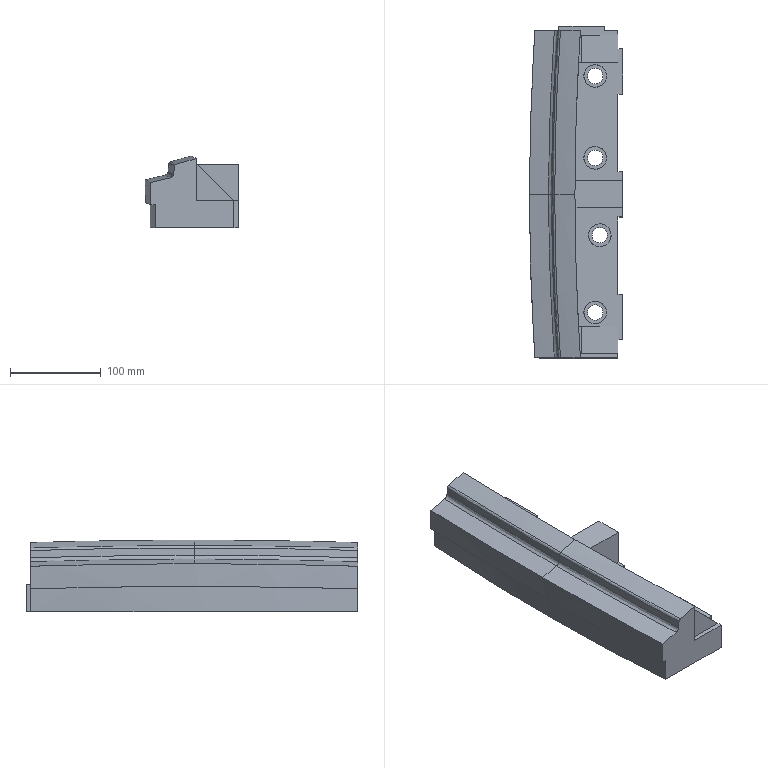Part | NX | features solid 2 | 1 solid | 65 faces | box 102.304 x 365 x 78.834 mm | volume 1719546 mm3 | plane 29 | spline 28 | cylinder 8 | commonest cylinder face diameters 17 x4 25 x4